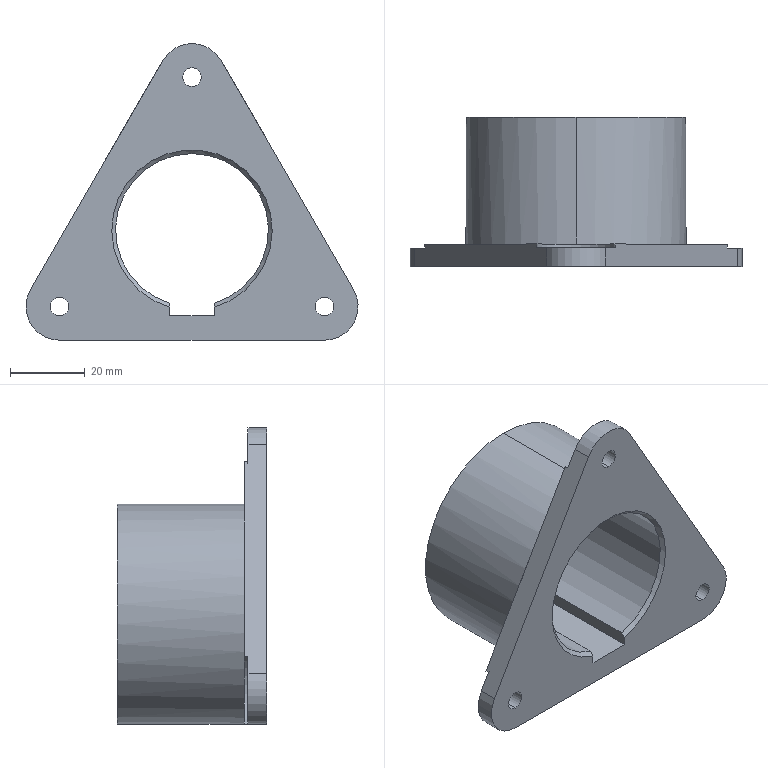Part | SolidWorks | features ICE 2, Chamfer 1, Extrusion 1, HoleWzd 1 | 1 solid | 34 faces | box 89.014 x 40 x 79.5 mm | volume 63655 mm3 | cylinder 17 | plane 14 | cone 3 | commonest cylinder face diameters 5 x6 21 x5 18 x3 59 x2 41 x1
STEP:
#1=CARTESIAN_POINT('',(35.507,5.,-10.));
#2=VERTEX_POINT('',#1);
#3=CARTESIAN_POINT('',(40.597,5.,-11.316));
#4=VERTEX_POINT('',#3);
#5=CARTESIAN_POINT('',(35.507,5.,-20.5));
#6=DIRECTION('',(0.,1.,0.));
#7=DIRECTION('',(0.,0.,1.));
#8=AXIS2_PLACEMENT_3D('',#5,#6,#7);
#9=CIRCLE('',#8,10.5);
#10=EDGE_CURVE('',#2,#4,#9,.T.);
#11=ORIENTED_EDGE('',*,*,#10,.F.);
#12=CARTESIAN_POINT('',(35.507,6.,-10.));
#13=VERTEX_POINT('',#12);
#14=CARTESIAN_POINT('',(35.507,5.,-10.));
#15=DIRECTION('',(0.,1.,0.));
#16=VECTOR('',#15,1000.);
#17=LINE('',#14,#16);
#18=EDGE_CURVE('',#2,#13,#17,.T.);
#19=ORIENTED_EDGE('',*,*,#18,.T.);
#20=CARTESIAN_POINT('',(40.597,6.,-11.316));
#21=VERTEX_POINT('',#20);
#22=CARTESIAN_POINT('',(35.507,6.,-20.5));
#23=DIRECTION('',(0.,1.,0.));
#24=DIRECTION('',(0.,0.,1.));
#25=AXIS2_PLACEMENT_3D('',#22,#23,#24);
#26=CIRCLE('',#25,10.5);
#27=EDGE_CURVE('',#13,#21,#26,.T.);
#28=ORIENTED_EDGE('',*,*,#27,.T.);
#29=CARTESIAN_POINT('',(40.597,5.,-11.316));
#30=DIRECTION('',(0.,-1.,0.));
#31=VECTOR('',#30,1000.);
#32=LINE('',#29,#31);
#33=EDGE_CURVE('',#21,#4,#32,.T.);
#34=ORIENTED_EDGE('',*,*,#33,.T.);
#35=EDGE_LOOP('',(#11,#19,#28,#34));
#36=FACE_OUTER_BOUND('',#35,.T.);
#37=CARTESIAN_POINT('',(35.507,5.,-20.5));
#38=DIRECTION('',(0.,1.,0.));
#39=DIRECTION('',(0.,0.,1.));
#40=AXIS2_PLACEMENT_3D('',#37,#38,#39);
#41=CYLINDRICAL_SURFACE('',#40,10.5);
#42=ADVANCED_FACE('',(#36),#41,.F.);
#43=CARTESIAN_POINT('',(-35.507,5.,-10.));
#44=VERTEX_POINT('',#43);
#45=CARTESIAN_POINT('',(-30.099,5.,-29.5));
#46=VERTEX_POINT('',#45);
#47=CARTESIAN_POINT('',(-35.507,5.,-20.5));
#48=DIRECTION('',(0.,1.,0.));
#49=DIRECTION('',(0.,0.,1.));
#50=AXIS2_PLACEMENT_3D('',#47,#48,#49);
#51=CIRCLE('',#50,10.5);
#52=EDGE_CURVE('',#44,#46,#51,.T.);
#53=ORIENTED_EDGE('',*,*,#52,.F.);
#54=CARTESIAN_POINT('',(-35.507,6.,-10.));
#55=VERTEX_POINT('',#54);
#56=CARTESIAN_POINT('',(-35.507,5.,-10.));
#57=DIRECTION('',(0.,1.,0.));
#58=VECTOR('',#57,1000.);
#59=LINE('',#56,#58);
#60=EDGE_CURVE('',#44,#55,#59,.T.);
#61=ORIENTED_EDGE('',*,*,#60,.T.);
#62=CARTESIAN_POINT('',(-30.099,6.,-29.5));
#63=VERTEX_POINT('',#62);
#64=CARTESIAN_POINT('',(-35.507,6.,-20.5));
#65=DIRECTION('',(0.,1.,0.));
#66=DIRECTION('',(0.,0.,1.));
#67=AXIS2_PLACEMENT_3D('',#64,#65,#66);
#68=CIRCLE('',#67,10.5);
#69=EDGE_CURVE('',#55,#63,#68,.T.);
#70=ORIENTED_EDGE('',*,*,#69,.T.);
#71=CARTESIAN_POINT('',(-30.099,5.,-29.5));
#72=DIRECTION('',(0.,-1.,0.));
#73=VECTOR('',#72,1000.);
#74=LINE('',#71,#73);
#75=EDGE_CURVE('',#63,#46,#74,.T.);
#76=ORIENTED_EDGE('',*,*,#75,.T.);
#77=EDGE_LOOP('',(#53,#61,#70,#76));
#78=FACE_OUTER_BOUND('',#77,.T.);
#79=CARTESIAN_POINT('',(-35.507,5.,-20.5));
#80=DIRECTION('',(0.,1.,0.));
#81=DIRECTION('',(0.,0.,1.));
#82=AXIS2_PLACEMENT_3D('',#79,#80,#81);
#83=CYLINDRICAL_SURFACE('',#82,10.5);
#84=ADVANCED_FACE('',(#78),#83,.F.);
#85=CARTESIAN_POINT('',(0.,39.,20.5));
#86=VERTEX_POINT('',#85);
#87=CARTESIAN_POINT('',(6.,39.,-19.602));
#88=VERTEX_POINT('',#87);
#89=CARTESIAN_POINT('',(0.,39.,0.));
#90=DIRECTION('',(0.,1.,0.));
#91=DIRECTION('',(0.,0.,1.));
#92=AXIS2_PLACEMENT_3D('',#89,#90,#91);
#93=CIRCLE('',#92,20.5);
#94=EDGE_CURVE('',#86,#88,#93,.T.);
#95=ORIENTED_EDGE('',*,*,#94,.F.);
#96=CARTESIAN_POINT('',(0.,40.,21.5));
#97=VERTEX_POINT('',#96);
#98=CARTESIAN_POINT('',(0.,39.,20.5));
#99=DIRECTION('',(0.,0.7071,0.7071));
#100=VECTOR('',#99,1000.);
#101=LINE('',#98,#100);
#102=EDGE_CURVE('',#86,#97,#101,.T.);
#103=ORIENTED_EDGE('',*,*,#102,.T.);
#104=CARTESIAN_POINT('',(6.,40.,-20.646));
#105=VERTEX_POINT('',#104);
#106=CARTESIAN_POINT('',(0.,40.,0.));
#107=DIRECTION('',(0.,-1.,0.));
#108=DIRECTION('',(0.,0.,1.));
#109=AXIS2_PLACEMENT_3D('',#106,#107,#108);
#110=CIRCLE('',#109,21.5);
#111=EDGE_CURVE('',#105,#97,#110,.T.);
#112=ORIENTED_EDGE('',*,*,#111,.F.);
#113=CARTESIAN_POINT('',(6.,39.,-19.602));
#114=CARTESIAN_POINT('',(6.,39.333,-19.95));
#115=CARTESIAN_POINT('',(6.,39.666,-20.298));
#116=CARTESIAN_POINT('',(6.,40.,-20.646));
#117=B_SPLINE_CURVE_WITH_KNOTS('',3,(#113,#114,#115,#116),.UNSPECIFIED.,.F.,.F.,(4,4),(0.,0.001445),.UNSPECIFIED.);
#118=EDGE_CURVE('',#88,#105,#117,.T.);
#119=ORIENTED_EDGE('',*,*,#118,.F.);
#120=EDGE_LOOP('',(#95,#103,#112,#119));
#121=FACE_OUTER_BOUND('',#120,.T.);
#122=CARTESIAN_POINT('',(0.,39.,0.));
#123=DIRECTION('',(0.,1.,0.));
#124=DIRECTION('',(0.,0.,1.));
#125=AXIS2_PLACEMENT_3D('',#122,#123,#124);
#126=CONICAL_SURFACE('',#125,20.5,0.7854);
#127=ADVANCED_FACE('',(#121),#126,.F.);
#128=CARTESIAN_POINT('',(0.,40.,29.5));
#129=VERTEX_POINT('',#128);
#130=CARTESIAN_POINT('',(0.,40.,-29.5));
#131=VERTEX_POINT('',#130);
#132=CARTESIAN_POINT('',(0.,40.,0.));
#133=DIRECTION('',(0.,1.,0.));
#134=DIRECTION('',(0.,0.,1.));
#135=AXIS2_PLACEMENT_3D('',#132,#133,#134);
#136=CIRCLE('',#135,29.5);
#137=EDGE_CURVE('',#129,#131,#136,.T.);
#138=ORIENTED_EDGE('',*,*,#137,.F.);
#139=CARTESIAN_POINT('',(0.,6.,29.5));
#140=VERTEX_POINT('',#139);
#141=CARTESIAN_POINT('',(0.,40.,29.5));
#142=DIRECTION('',(0.,-1.,0.));
#143=VECTOR('',#142,1000.);
#144=LINE('',#141,#143);
#145=EDGE_CURVE('',#129,#140,#144,.T.);
#146=ORIENTED_EDGE('',*,*,#145,.T.);
#147=CARTESIAN_POINT('',(25.548,6.,14.75));
#148=VERTEX_POINT('',#147);
#149=CARTESIAN_POINT('',(0.,6.,0.));
#150=DIRECTION('',(0.,1.,0.));
#151=DIRECTION('',(0.,0.,1.));
#152=AXIS2_PLACEMENT_3D('',#149,#150,#151);
#153=CIRCLE('',#152,29.5);
#154=EDGE_CURVE('',#140,#148,#153,.T.);
#155=ORIENTED_EDGE('',*,*,#154,.T.);
#156=CARTESIAN_POINT('',(0.,6.,-29.5));
#157=VERTEX_POINT('',#156);
#158=CARTESIAN_POINT('',(0.,6.,0.));
#159=DIRECTION('',(0.,1.,0.));
#160=DIRECTION('',(0.,0.,1.));
#161=AXIS2_PLACEMENT_3D('',#158,#159,#160);
#162=CIRCLE('',#161,29.5);
#163=EDGE_CURVE('',#148,#157,#162,.T.);
#164=ORIENTED_EDGE('',*,*,#163,.T.);
#165=CARTESIAN_POINT('',(0.,40.,-29.5));
#166=DIRECTION('',(0.,-1.,0.));
#167=VECTOR('',#166,1000.);
#168=LINE('',#165,#167);
#169=EDGE_CURVE('',#131,#157,#168,.T.);
#170=ORIENTED_EDGE('',*,*,#169,.F.);
#171=EDGE_LOOP('',(#138,#146,#155,#164,#170));
#172=FACE_OUTER_BOUND('',#171,.T.);
#173=CARTESIAN_POINT('',(0.,40.,0.));
#174=DIRECTION('',(0.,-1.,0.));
#175=DIRECTION('',(0.,0.,-1.));
#176=AXIS2_PLACEMENT_3D('',#173,#174,#175);
#177=CYLINDRICAL_SURFACE('',#176,29.5);
#178=ADVANCED_FACE('',(#172),#177,.T.);
#179=CARTESIAN_POINT('',(-35.507,0.,-23.));
#180=VERTEX_POINT('',#179);
#181=CARTESIAN_POINT('',(-35.507,0.,-18.));
#182=VERTEX_POINT('',#181);
#183=CARTESIAN_POINT('',(-35.507,0.,-20.5));
#184=DIRECTION('',(0.,1.,0.));
#185=DIRECTION('',(0.,0.,1.));
#186=AXIS2_PLACEMENT_3D('',#183,#184,#185);
#187=CIRCLE('',#186,2.5);
#188=EDGE_CURVE('',#180,#182,#187,.T.);
#189=ORIENTED_EDGE('',*,*,#188,.F.);
#190=CARTESIAN_POINT('',(-35.507,5.,-23.));
#191=VERTEX_POINT('',#190);
#192=CARTESIAN_POINT('',(-35.507,6.,-23.));
#193=DIRECTION('',(0.,1.,0.));
#194=VECTOR('',#193,1000.);
#195=LINE('',#192,#194);
#196=EDGE_CURVE('',#180,#191,#195,.T.);
#197=ORIENTED_EDGE('',*,*,#196,.T.);
#198=CARTESIAN_POINT('',(-35.507,5.,-18.));
#199=VERTEX_POINT('',#198);
#200=CARTESIAN_POINT('',(-35.507,5.,-20.5));
#201=DIRECTION('',(0.,-1.,0.));
#202=DIRECTION('',(0.,0.,1.));
#203=AXIS2_PLACEMENT_3D('',#200,#201,#202);
#204=CIRCLE('',#203,2.5);
#205=EDGE_CURVE('',#199,#191,#204,.T.);
#206=ORIENTED_EDGE('',*,*,#205,.F.);
#207=CARTESIAN_POINT('',(-35.507,6.,-18.));
#208=DIRECTION('',(0.,1.,0.));
#209=VECTOR('',#208,1000.);
#210=LINE('',#207,#209);
#211=EDGE_CURVE('',#182,#199,#210,.T.);
#212=ORIENTED_EDGE('',*,*,#211,.F.);
#213=EDGE_LOOP('',(#189,#197,#206,#212));
#214=FACE_OUTER_BOUND('',#213,.T.);
#215=CARTESIAN_POINT('',(-35.507,6.,-20.5));
#216=DIRECTION('',(0.,1.,0.));
#217=DIRECTION('',(0.,0.,1.));
#218=AXIS2_PLACEMENT_3D('',#215,#216,#217);
#219=CYLINDRICAL_SURFACE('',#218,2.5);
#220=ADVANCED_FACE('',(#214),#219,.F.);
#221=CARTESIAN_POINT('',(35.507,0.,-23.));
#222=VERTEX_POINT('',#221);
#223=CARTESIAN_POINT('',(35.507,0.,-18.));
#224=VERTEX_POINT('',#223);
#225=CARTESIAN_POINT('',(35.507,0.,-20.5));
#226=DIRECTION('',(0.,1.,0.));
#227=DIRECTION('',(0.,0.,1.));
#228=AXIS2_PLACEMENT_3D('',#225,#226,#227);
#229=CIRCLE('',#228,2.5);
#230=EDGE_CURVE('',#222,#224,#229,.T.);
#231=ORIENTED_EDGE('',*,*,#230,.F.);
#232=CARTESIAN_POINT('',(35.507,5.,-23.));
#233=VERTEX_POINT('',#232);
#234=CARTESIAN_POINT('',(35.507,6.,-23.));
#235=DIRECTION('',(0.,1.,0.));
#236=VECTOR('',#235,1000.);
#237=LINE('',#234,#236);
#238=EDGE_CURVE('',#222,#233,#237,.T.);
#239=ORIENTED_EDGE('',*,*,#238,.T.);
#240=CARTESIAN_POINT('',(35.507,5.,-18.));
#241=VERTEX_POINT('',#240);
#242=CARTESIAN_POINT('',(35.507,5.,-20.5));
#243=DIRECTION('',(0.,-1.,0.));
#244=DIRECTION('',(0.,0.,1.));
#245=AXIS2_PLACEMENT_3D('',#242,#243,#244);
#246=CIRCLE('',#245,2.5);
#247=EDGE_CURVE('',#241,#233,#246,.T.);
#248=ORIENTED_EDGE('',*,*,#247,.F.);
#249=CARTESIAN_POINT('',(35.507,6.,-18.));
#250=DIRECTION('',(0.,1.,0.));
#251=VECTOR('',#250,1000.);
#252=LINE('',#249,#251);
#253=EDGE_CURVE('',#224,#241,#252,.T.);
#254=ORIENTED_EDGE('',*,*,#253,.F.);
#255=EDGE_LOOP('',(#231,#239,#248,#254));
#256=FACE_OUTER_BOUND('',#255,.T.);
#257=CARTESIAN_POINT('',(35.507,6.,-20.5));
#258=DIRECTION('',(0.,1.,0.));
#259=DIRECTION('',(0.,0.,1.));
#260=AXIS2_PLACEMENT_3D('',#257,#258,#259);
#261=CYLINDRICAL_SURFACE('',#260,2.5);
#262=ADVANCED_FACE('',(#256),#261,.F.);
#263=CARTESIAN_POINT('',(0.,0.,38.5));
#264=VERTEX_POINT('',#263);
#265=CARTESIAN_POINT('',(0.,0.,43.5));
#266=VERTEX_POINT('',#265);
#267=CARTESIAN_POINT('',(0.,0.,41.));
#268=DIRECTION('',(0.,1.,0.));
#269=DIRECTION('',(0.,0.,1.));
#270=AXIS2_PLACEMENT_3D('',#267,#268,#269);
#271=CIRCLE('',#270,2.5);
#272=EDGE_CURVE('',#264,#266,#271,.T.);
#273=ORIENTED_EDGE('',*,*,#272,.F.);
#274=CARTESIAN_POINT('',(0.,5.,38.5));
#275=VERTEX_POINT('',#274);
#276=CARTESIAN_POINT('',(0.,6.,38.5));
#277=DIRECTION('',(0.,1.,0.));
#278=VECTOR('',#277,1000.);
#279=LINE('',#276,#278);
#280=EDGE_CURVE('',#264,#275,#279,.T.);
#281=ORIENTED_EDGE('',*,*,#280,.T.);
#282=CARTESIAN_POINT('',(0.,5.,43.5));
#283=VERTEX_POINT('',#282);
#284=CARTESIAN_POINT('',(0.,5.,41.));
#285=DIRECTION('',(0.,-1.,0.));
#286=DIRECTION('',(0.,0.,1.));
#287=AXIS2_PLACEMENT_3D('',#284,#285,#286);
#288=CIRCLE('',#287,2.5);
#289=EDGE_CURVE('',#283,#275,#288,.T.);
#290=ORIENTED_EDGE('',*,*,#289,.F.);
#291=CARTESIAN_POINT('',(0.,6.,43.5));
#292=DIRECTION('',(0.,1.,0.));
#293=VECTOR('',#292,1000.);
#294=LINE('',#291,#293);
#295=EDGE_CURVE('',#266,#283,#294,.T.);
#296=ORIENTED_EDGE('',*,*,#295,.F.);
#297=EDGE_LOOP('',(#273,#281,#290,#296));
#298=FACE_OUTER_BOUND('',#297,.T.);
#299=CARTESIAN_POINT('',(0.,6.,41.));
#300=DIRECTION('',(0.,1.,0.));
#301=DIRECTION('',(0.,0.,1.));
#302=AXIS2_PLACEMENT_3D('',#299,#300,#301);
#303=CYLINDRICAL_SURFACE('',#302,2.5);
#304=ADVANCED_FACE('',(#298),#303,.F.);
#305=CARTESIAN_POINT('',(-7.794,5.,45.5));
#306=VERTEX_POINT('',#305);
#307=CARTESIAN_POINT('',(7.794,5.,45.5));
#308=VERTEX_POINT('',#307);
#309=CARTESIAN_POINT('',(0.,5.,41.));
#310=DIRECTION('',(0.,1.,0.));
#311=DIRECTION('',(0.,0.,1.));
#312=AXIS2_PLACEMENT_3D('',#309,#310,#311);
#313=CIRCLE('',#312,9.);
#314=EDGE_CURVE('',#306,#308,#313,.T.);
#315=ORIENTED_EDGE('',*,*,#314,.F.);
#316=CARTESIAN_POINT('',(-7.794,0.,45.5));
#317=VERTEX_POINT('',#316);
#318=CARTESIAN_POINT('',(-7.794,6.,45.5));
#319=DIRECTION('',(0.,-1.,0.));
#320=VECTOR('',#319,1000.);
#321=LINE('',#318,#320);
#322=EDGE_CURVE('',#306,#317,#321,.T.);
#323=ORIENTED_EDGE('',*,*,#322,.T.);
#324=CARTESIAN_POINT('',(7.794,0.,45.5));
#325=VERTEX_POINT('',#324);
#326=CARTESIAN_POINT('',(0.,0.,41.));
#327=DIRECTION('',(0.,1.,0.));
#328=DIRECTION('',(0.,0.,1.));
#329=AXIS2_PLACEMENT_3D('',#326,#327,#328);
#330=CIRCLE('',#329,9.);
#331=EDGE_CURVE('',#317,#325,#330,.T.);
#332=ORIENTED_EDGE('',*,*,#331,.T.);
#333=CARTESIAN_POINT('',(7.794,6.,45.5));
#334=DIRECTION('',(0.,-1.,0.));
#335=VECTOR('',#334,1000.);
#336=LINE('',#333,#335);
#337=EDGE_CURVE('',#308,#325,#336,.T.);
#338=ORIENTED_EDGE('',*,*,#337,.F.);
#339=EDGE_LOOP('',(#315,#323,#332,#338));
#340=FACE_OUTER_BOUND('',#339,.T.);
#341=CARTESIAN_POINT('',(0.,6.,41.));
#342=DIRECTION('',(0.,-1.,0.));
#343=DIRECTION('',(0.,0.,-1.));
#344=AXIS2_PLACEMENT_3D('',#341,#342,#343);
#345=CYLINDRICAL_SURFACE('',#344,9.);
#346=ADVANCED_FACE('',(#340),#345,.T.);
#347=ORIENTED_EDGE('',*,*,#280,.F.);
#348=CARTESIAN_POINT('',(0.,0.,41.));
#349=DIRECTION('',(0.,1.,0.));
#350=DIRECTION('',(0.,0.,1.));
#351=AXIS2_PLACEMENT_3D('',#348,#349,#350);
#352=CIRCLE('',#351,2.5);
#353=EDGE_CURVE('',#266,#264,#352,.T.);
#354=ORIENTED_EDGE('',*,*,#353,.F.);
#355=ORIENTED_EDGE('',*,*,#295,.T.);
#356=CARTESIAN_POINT('',(0.,5.,41.));
#357=DIRECTION('',(0.,-1.,0.));
#358=DIRECTION('',(0.,0.,1.));
#359=AXIS2_PLACEMENT_3D('',#356,#357,#358);
#360=CIRCLE('',#359,2.5);
#361=EDGE_CURVE('',#275,#283,#360,.T.);
#362=ORIENTED_EDGE('',*,*,#361,.F.);
#363=EDGE_LOOP('',(#347,#354,#355,#362));
#364=FACE_OUTER_BOUND('',#363,.T.);
#365=CARTESIAN_POINT('',(0.,6.,41.));
#366=DIRECTION('',(0.,1.,0.));
#367=DIRECTION('',(0.,0.,1.));
#368=AXIS2_PLACEMENT_3D('',#365,#366,#367);
#369=CYLINDRICAL_SURFACE('',#368,2.5);
#370=ADVANCED_FACE('',(#364),#369,.F.);
#371=CARTESIAN_POINT('',(43.301,5.,-16.));
#372=VERTEX_POINT('',#371);
#373=CARTESIAN_POINT('',(35.507,5.,-29.5));
#374=VERTEX_POINT('',#373);
#375=CARTESIAN_POINT('',(35.507,5.,-20.5));
#376=DIRECTION('',(0.,1.,0.));
#377=DIRECTION('',(0.,0.,1.));
#378=AXIS2_PLACEMENT_3D('',#375,#376,#377);
#379=CIRCLE('',#378,9.);
#380=EDGE_CURVE('',#372,#374,#379,.T.);
#381=ORIENTED_EDGE('',*,*,#380,.F.);
#382=CARTESIAN_POINT('',(43.301,0.,-16.));
#383=VERTEX_POINT('',#382);
#384=CARTESIAN_POINT('',(43.301,6.,-16.));
#385=DIRECTION('',(0.,-1.,0.));
#386=VECTOR('',#385,1000.);
#387=LINE('',#384,#386);
#388=EDGE_CURVE('',#372,#383,#387,.T.);
#389=ORIENTED_EDGE('',*,*,#388,.T.);
#390=CARTESIAN_POINT('',(35.507,0.,-29.5));
#391=VERTEX_POINT('',#390);
#392=CARTESIAN_POINT('',(35.507,0.,-20.5));
#393=DIRECTION('',(0.,1.,0.));
#394=DIRECTION('',(0.,0.,1.));
#395=AXIS2_PLACEMENT_3D('',#392,#393,#394);
#396=CIRCLE('',#395,9.);
#397=EDGE_CURVE('',#383,#391,#396,.T.);
#398=ORIENTED_EDGE('',*,*,#397,.T.);
#399=CARTESIAN_POINT('',(35.507,6.,-29.5));
#400=DIRECTION('',(0.,-1.,0.));
#401=VECTOR('',#400,1000.);
#402=LINE('',#399,#401);
#403=EDGE_CURVE('',#374,#391,#402,.T.);
#404=ORIENTED_EDGE('',*,*,#403,.F.);
#405=EDGE_LOOP('',(#381,#389,#398,#404));
#406=FACE_OUTER_BOUND('',#405,.T.);
#407=CARTESIAN_POINT('',(35.507,6.,-20.5));
#408=DIRECTION('',(0.,-1.,0.));
#409=DIRECTION('',(0.,0.,-1.));
#410=AXIS2_PLACEMENT_3D('',#407,#408,#409);
#411=CYLINDRICAL_SURFACE('',#410,9.);
#412=ADVANCED_FACE('',(#406),#411,.T.);
#413=ORIENTED_EDGE('',*,*,#238,.F.);
#414=CARTESIAN_POINT('',(35.507,0.,-20.5));
#415=DIRECTION('',(0.,1.,0.));
#416=DIRECTION('',(0.,0.,1.));
#417=AXIS2_PLACEMENT_3D('',#414,#415,#416);
#418=CIRCLE('',#417,2.5);
#419=EDGE_CURVE('',#224,#222,#418,.T.);
#420=ORIENTED_EDGE('',*,*,#419,.F.);
#421=ORIENTED_EDGE('',*,*,#253,.T.);
#422=CARTESIAN_POINT('',(35.507,5.,-20.5));
#423=DIRECTION('',(0.,-1.,0.));
#424=DIRECTION('',(0.,0.,1.));
#425=AXIS2_PLACEMENT_3D('',#422,#423,#424);
#426=CIRCLE('',#425,2.5);
#427=EDGE_CURVE('',#233,#241,#426,.T.);
#428=ORIENTED_EDGE('',*,*,#427,.F.);
#429=EDGE_LOOP('',(#413,#420,#421,#428));
#430=FACE_OUTER_BOUND('',#429,.T.);
#431=CARTESIAN_POINT('',(35.507,6.,-20.5));
#432=DIRECTION('',(0.,1.,0.));
#433=DIRECTION('',(0.,0.,1.));
#434=AXIS2_PLACEMENT_3D('',#431,#432,#433);
#435=CYLINDRICAL_SURFACE('',#434,2.5);
#436=ADVANCED_FACE('',(#430),#435,.F.);
#437=CARTESIAN_POINT('',(-35.507,5.,-29.5));
#438=VERTEX_POINT('',#437);
#439=CARTESIAN_POINT('',(-43.301,5.,-16.));
#440=VERTEX_POINT('',#439);
#441=CARTESIAN_POINT('',(-35.507,5.,-20.5));
#442=DIRECTION('',(0.,1.,0.));
#443=DIRECTION('',(0.,0.,1.));
#444=AXIS2_PLACEMENT_3D('',#441,#442,#443);
#445=CIRCLE('',#444,9.);
#446=EDGE_CURVE('',#438,#440,#445,.T.);
#447=ORIENTED_EDGE('',*,*,#446,.F.);
#448=CARTESIAN_POINT('',(-35.507,0.,-29.5));
#449=VERTEX_POINT('',#448);
#450=CARTESIAN_POINT('',(-35.507,6.,-29.5));
#451=DIRECTION('',(0.,-1.,0.));
#452=VECTOR('',#451,1000.);
#453=LINE('',#450,#452);
#454=EDGE_CURVE('',#438,#449,#453,.T.);
#455=ORIENTED_EDGE('',*,*,#454,.T.);
#456=CARTESIAN_POINT('',(-43.301,0.,-16.));
#457=VERTEX_POINT('',#456);
#458=CARTESIAN_POINT('',(-35.507,0.,-20.5));
#459=DIRECTION('',(0.,1.,0.));
#460=DIRECTION('',(0.,0.,1.));
#461=AXIS2_PLACEMENT_3D('',#458,#459,#460);
#462=CIRCLE('',#461,9.);
#463=EDGE_CURVE('',#449,#457,#462,.T.);
#464=ORIENTED_EDGE('',*,*,#463,.T.);
#465=CARTESIAN_POINT('',(-43.301,6.,-16.));
#466=DIRECTION('',(0.,-1.,0.));
#467=VECTOR('',#466,1000.);
#468=LINE('',#465,#467);
#469=EDGE_CURVE('',#440,#457,#468,.T.);
#470=ORIENTED_EDGE('',*,*,#469,.F.);
#471=EDGE_LOOP('',(#447,#455,#464,#470));
#472=FACE_OUTER_BOUND('',#471,.T.);
#473=CARTESIAN_POINT('',(-35.507,6.,-20.5));
#474=DIRECTION('',(0.,-1.,0.));
#475=DIRECTION('',(0.,0.,-1.));
#476=AXIS2_PLACEMENT_3D('',#473,#474,#475);
#477=CYLINDRICAL_SURFACE('',#476,9.);
#478=ADVANCED_FACE('',(#472),#477,.T.);
#479=ORIENTED_EDGE('',*,*,#196,.F.);
#480=CARTESIAN_POINT('',(-35.507,0.,-20.5));
#481=DIRECTION('',(0.,1.,0.));
#482=DIRECTION('',(0.,0.,1.));
#483=AXIS2_PLACEMENT_3D('',#480,#481,#482);
#484=CIRCLE('',#483,2.5);
#485=EDGE_CURVE('',#182,#180,#484,.T.);
#486=ORIENTED_EDGE('',*,*,#485,.F.);
#487=ORIENTED_EDGE('',*,*,#211,.T.);
#488=CARTESIAN_POINT('',(-35.507,5.,-20.5));
#489=DIRECTION('',(0.,-1.,0.));
#490=DIRECTION('',(0.,0.,1.));
#491=AXIS2_PLACEMENT_3D('',#488,#489,#490);
#492=CIRCLE('',#491,2.5);
#493=EDGE_CURVE('',#191,#199,#492,.T.);
#494=ORIENTED_EDGE('',*,*,#493,.F.);
#495=EDGE_LOOP('',(#479,#486,#487,#494));
#496=FACE_OUTER_BOUND('',#495,.T.);
#497=CARTESIAN_POINT('',(-35.507,6.,-20.5));
#498=DIRECTION('',(0.,1.,0.));
#499=DIRECTION('',(0.,0.,1.));
#500=AXIS2_PLACEMENT_3D('',#497,#498,#499);
#501=CYLINDRICAL_SURFACE('',#500,2.5);
#502=ADVANCED_FACE('',(#496),#501,.F.);
#503=CARTESIAN_POINT('',(30.099,5.,-29.5));
#504=VERTEX_POINT('',#503);
#505=CARTESIAN_POINT('',(30.099,6.,-29.5));
#506=VERTEX_POINT('',#505);
#507=CARTESIAN_POINT('',(30.099,5.,-29.5));
#508=DIRECTION('',(0.,1.,0.));
#509=VECTOR('',#508,1000.);
#510=LINE('',#507,#509);
#511=EDGE_CURVE('',#504,#506,#510,.T.);
#512=ORIENTED_EDGE('',*,*,#511,.F.);
#513=CARTESIAN_POINT('',(0.,5.,-29.5));
#514=DIRECTION('',(1.,0.,0.));
#515=VECTOR('',#514,1000.);
#516=LINE('',#513,#515);
#517=EDGE_CURVE('',#504,#374,#516,.T.);
#518=ORIENTED_EDGE('',*,*,#517,.T.);
#519=ORIENTED_EDGE('',*,*,#403,.T.);
#520=CARTESIAN_POINT('',(0.,0.,-29.5));
#521=DIRECTION('',(1.,0.,0.));
#522=VECTOR('',#521,1000.);
#523=LINE('',#520,#522);
#524=EDGE_CURVE('',#449,#391,#523,.T.);
#525=ORIENTED_EDGE('',*,*,#524,.F.);
#526=ORIENTED_EDGE('',*,*,#454,.F.);
#527=CARTESIAN_POINT('',(0.,5.,-29.5));
#528=DIRECTION('',(1.,0.,0.));
#529=VECTOR('',#528,1000.);
#530=LINE('',#527,#529);
#531=EDGE_CURVE('',#438,#46,#530,.T.);
#532=ORIENTED_EDGE('',*,*,#531,.T.);
#533=ORIENTED_EDGE('',*,*,#75,.F.);
#534=CARTESIAN_POINT('',(0.,6.,-29.5));
#535=DIRECTION('',(1.,0.,0.));
#536=VECTOR('',#535,1000.);
#537=LINE('',#534,#536);
#538=EDGE_CURVE('',#63,#157,#537,.T.);
#539=ORIENTED_EDGE('',*,*,#538,.T.);
#540=CARTESIAN_POINT('',(0.,6.,-29.5));
#541=DIRECTION('',(1.,0.,0.));
#542=VECTOR('',#541,1000.);
#543=LINE('',#540,#542);
#544=EDGE_CURVE('',#157,#506,#543,.T.);
#545=ORIENTED_EDGE('',*,*,#544,.T.);
#546=EDGE_LOOP('',(#512,#518,#519,#525,#526,#532,#533,#539,#545));
#547=FACE_OUTER_BOUND('',#546,.T.);
#548=CARTESIAN_POINT('',(0.,6.,-29.5));
#549=DIRECTION('',(0.,0.,-1.));
#550=DIRECTION('',(-1.,0.,0.));
#551=AXIS2_PLACEMENT_3D('',#548,#549,#550);
#552=PLANE('',#551);
#553=ADVANCED_FACE('',(#547),#552,.T.);
#554=CARTESIAN_POINT('',(-10.498,6.,40.816));
#555=VERTEX_POINT('',#554);
#556=CARTESIAN_POINT('',(-10.498,5.,40.816));
#557=VERTEX_POINT('',#556);
#558=CARTESIAN_POINT('',(-10.498,5.,40.816));
#559=DIRECTION('',(0.,-1.,0.));
#560=VECTOR('',#559,1000.);
#561=LINE('',#558,#560);
#562=EDGE_CURVE('',#555,#557,#561,.T.);
#563=ORIENTED_EDGE('',*,*,#562,.F.);
#564=CARTESIAN_POINT('',(-25.548,6.,14.75));
#565=VERTEX_POINT('',#564);
#566=CARTESIAN_POINT('',(-25.548,6.,14.75));
#567=DIRECTION('',(-0.5,0.,-0.866));
#568=VECTOR('',#567,1000.);
#569=LINE('',#566,#568);
#570=EDGE_CURVE('',#555,#565,#569,.T.);
#571=ORIENTED_EDGE('',*,*,#570,.T.);
#572=CARTESIAN_POINT('',(-40.597,6.,-11.316));
#573=VERTEX_POINT('',#572);
#574=CARTESIAN_POINT('',(-25.548,6.,14.75));
#575=DIRECTION('',(-0.5,0.,-0.866));
#576=VECTOR('',#575,1000.);
#577=LINE('',#574,#576);
#578=EDGE_CURVE('',#565,#573,#577,.T.);
#579=ORIENTED_EDGE('',*,*,#578,.T.);
#580=CARTESIAN_POINT('',(-40.597,5.,-11.316));
#581=VERTEX_POINT('',#580);
#582=CARTESIAN_POINT('',(-40.597,5.,-11.316));
#583=DIRECTION('',(0.,1.,0.));
#584=VECTOR('',#583,1000.);
#585=LINE('',#582,#584);
#586=EDGE_CURVE('',#581,#573,#585,.T.);
#587=ORIENTED_EDGE('',*,*,#586,.F.);
#588=CARTESIAN_POINT('',(-25.548,5.,14.75));
#589=DIRECTION('',(-0.5,0.,-0.866));
#590=VECTOR('',#589,1000.);
#591=LINE('',#588,#590);
#592=EDGE_CURVE('',#581,#440,#591,.T.);
#593=ORIENTED_EDGE('',*,*,#592,.T.);
#594=ORIENTED_EDGE('',*,*,#469,.T.);
#595=CARTESIAN_POINT('',(-25.548,0.,14.75));
#596=DIRECTION('',(-0.5,0.,-0.866));
#597=VECTOR('',#596,1000.);
#598=LINE('',#595,#597);
#599=EDGE_CURVE('',#317,#457,#598,.T.);
#600=ORIENTED_EDGE('',*,*,#599,.F.);
#601=ORIENTED_EDGE('',*,*,#322,.F.);
#602=CARTESIAN_POINT('',(-25.548,5.,14.75));
#603=DIRECTION('',(-0.5,0.,-0.866));
#604=VECTOR('',#603,1000.);
#605=LINE('',#602,#604);
#606=EDGE_CURVE('',#306,#557,#605,.T.);
#607=ORIENTED_EDGE('',*,*,#606,.T.);
#608=EDGE_LOOP('',(#563,#571,#579,#587,#593,#594,#600,#601,#607));
#609=FACE_OUTER_BOUND('',#608,.T.);
#610=CARTESIAN_POINT('',(-25.548,6.,14.75));
#611=DIRECTION('',(-0.866,0.,0.5));
#612=DIRECTION('',(0.5,0.,0.866));
#613=AXIS2_PLACEMENT_3D('',#610,#611,#612);
#614=PLANE('',#613);
#615=ADVANCED_FACE('',(#609),#614,.T.);
#616=CARTESIAN_POINT('',(-35.507,6.,-20.5));
#617=DIRECTION('',(0.,1.,0.));
#618=DIRECTION('',(0.,0.,1.));
#619=AXIS2_PLACEMENT_3D('',#616,#617,#618);
#620=CIRCLE('',#619,10.5);
#621=EDGE_CURVE('',#573,#55,#620,.T.);
#622=ORIENTED_EDGE('',*,*,#621,.F.);
#623=ORIENTED_EDGE('',*,*,#578,.F.);
#624=CARTESIAN_POINT('',(0.,6.,0.));
#625=DIRECTION('',(0.,1.,0.));
#626=DIRECTION('',(0.,0.,1.));
#627=AXIS2_PLACEMENT_3D('',#624,#625,#626);
#628=CIRCLE('',#627,29.5);
#629=EDGE_CURVE('',#157,#565,#628,.T.);
#630=ORIENTED_EDGE('',*,*,#629,.F.);
#631=ORIENTED_EDGE('',*,*,#538,.F.);
#632=ORIENTED_EDGE('',*,*,#69,.F.);
#633=EDGE_LOOP('',(#622,#623,#630,#631,#632));
#634=FACE_OUTER_BOUND('',#633,.T.);
#635=CARTESIAN_POINT('',(0.,6.,0.));
#636=DIRECTION('',(0.,1.,0.));
#637=DIRECTION('',(0.,0.,1.));
#638=AXIS2_PLACEMENT_3D('',#635,#636,#637);
#639=PLANE('',#638);
#640=ADVANCED_FACE('',(#634),#639,.T.);
#641=ORIENTED_EDGE('',*,*,#485,.T.);
#642=ORIENTED_EDGE('',*,*,#188,.T.);
#643=EDGE_LOOP('',(#641,#642));
#644=FACE_BOUND('',#643,.T.);
#645=ORIENTED_EDGE('',*,*,#419,.T.);
#646=ORIENTED_EDGE('',*,*,#230,.T.);
#647=EDGE_LOOP('',(#645,#646));
#648=FACE_BOUND('',#647,.T.);
#649=ORIENTED_EDGE('',*,*,#353,.T.);
#650=ORIENTED_EDGE('',*,*,#272,.T.);
#651=EDGE_LOOP('',(#649,#650));
#652=FACE_BOUND('',#651,.T.);
#653=ORIENTED_EDGE('',*,*,#524,.T.);
#654=ORIENTED_EDGE('',*,*,#397,.F.);
#655=CARTESIAN_POINT('',(25.548,0.,14.75));
#656=DIRECTION('',(-0.5,0.,0.866));
#657=VECTOR('',#656,1000.);
#658=LINE('',#655,#657);
#659=EDGE_CURVE('',#383,#325,#658,.T.);
#660=ORIENTED_EDGE('',*,*,#659,.T.);
#661=ORIENTED_EDGE('',*,*,#331,.F.);
#662=ORIENTED_EDGE('',*,*,#599,.T.);
#663=ORIENTED_EDGE('',*,*,#463,.F.);
#664=EDGE_LOOP('',(#653,#654,#660,#661,#662,#663));
#665=FACE_OUTER_BOUND('',#664,.T.);
#666=CARTESIAN_POINT('',(-6.,0.,-22.902));
#667=VERTEX_POINT('',#666);
#668=CARTESIAN_POINT('',(-6.,0.,-20.646));
#669=VERTEX_POINT('',#668);
#670=CARTESIAN_POINT('',(-6.,0.,-22.902));
#671=DIRECTION('',(0.,0.,1.));
#672=VECTOR('',#671,1000.);
#673=LINE('',#670,#672);
#674=EDGE_CURVE('',#667,#669,#673,.T.);
#675=ORIENTED_EDGE('',*,*,#674,.T.);
#676=CARTESIAN_POINT('',(6.,0.,-20.646));
#677=VERTEX_POINT('',#676);
#678=CARTESIAN_POINT('',(0.,0.,0.));
#679=DIRECTION('',(0.,1.,0.));
#680=DIRECTION('',(0.,0.,1.));
#681=AXIS2_PLACEMENT_3D('',#678,#679,#680);
#682=CIRCLE('',#681,21.5);
#683=EDGE_CURVE('',#669,#677,#682,.T.);
#684=ORIENTED_EDGE('',*,*,#683,.T.);
#685=CARTESIAN_POINT('',(6.,0.,-22.902));
#686=VERTEX_POINT('',#685);
#687=CARTESIAN_POINT('',(6.,0.,-19.602));
#688=DIRECTION('',(0.,0.,-1.));
#689=VECTOR('',#688,1000.);
#690=LINE('',#687,#689);
#691=EDGE_CURVE('',#677,#686,#690,.T.);
#692=ORIENTED_EDGE('',*,*,#691,.T.);
#693=CARTESIAN_POINT('',(6.,0.,-22.902));
#694=DIRECTION('',(-1.,0.,0.));
#695=VECTOR('',#694,1000.);
#696=LINE('',#693,#695);
#697=EDGE_CURVE('',#686,#667,#696,.T.);
#698=ORIENTED_EDGE('',*,*,#697,.T.);
#699=EDGE_LOOP('',(#675,#684,#692,#698));
#700=FACE_BOUND('',#699,.T.);
#701=CARTESIAN_POINT('',(0.,0.,0.));
#702=DIRECTION('',(0.,1.,0.));
#703=DIRECTION('',(0.,0.,1.));
#704=AXIS2_PLACEMENT_3D('',#701,#702,#703);
#705=PLANE('',#704);
#706=ADVANCED_FACE('',(#644,#648,#652,#665,#700),#705,.F.);
#707=ORIENTED_EDGE('',*,*,#145,.F.);
#708=CARTESIAN_POINT('',(0.,40.,0.));
#709=DIRECTION('',(0.,1.,0.));
#710=DIRECTION('',(0.,0.,1.));
#711=AXIS2_PLACEMENT_3D('',#708,#709,#710);
#712=CIRCLE('',#711,29.5);
#713=EDGE_CURVE('',#131,#129,#712,.T.);
#714=ORIENTED_EDGE('',*,*,#713,.F.);
#715=ORIENTED_EDGE('',*,*,#169,.T.);
#716=ORIENTED_EDGE('',*,*,#629,.T.);
#717=CARTESIAN_POINT('',(0.,6.,0.));
#718=DIRECTION('',(0.,1.,0.));
#719=DIRECTION('',(0.,0.,1.));
#720=AXIS2_PLACEMENT_3D('',#717,#718,#719);
#721=CIRCLE('',#720,29.5);
#722=EDGE_CURVE('',#565,#140,#721,.T.);
#723=ORIENTED_EDGE('',*,*,#722,.T.);
#724=EDGE_LOOP('',(#707,#714,#715,#716,#723));
#725=FACE_OUTER_BOUND('',#724,.T.);
#726=CARTESIAN_POINT('',(0.,40.,0.));
#727=DIRECTION('',(0.,-1.,0.));
#728=DIRECTION('',(0.,0.,-1.));
#729=AXIS2_PLACEMENT_3D('',#726,#727,#728);
#730=CYLINDRICAL_SURFACE('',#729,29.5);
#731=ADVANCED_FACE('',(#725),#730,.T.);
#732=ORIENTED_EDGE('',*,*,#713,.T.);
#733=ORIENTED_EDGE('',*,*,#137,.T.);
#734=EDGE_LOOP('',(#732,#733));
#735=FACE_OUTER_BOUND('',#734,.T.);
#736=CARTESIAN_POINT('',(6.,40.,-22.902));
#737=VERTEX_POINT('',#736);
#738=CARTESIAN_POINT('',(6.,40.,-19.602));
#739=DIRECTION('',(0.,0.,-1.));
#740=VECTOR('',#739,1000.);
#741=LINE('',#738,#740);
#742=EDGE_CURVE('',#105,#737,#741,.T.);
#743=ORIENTED_EDGE('',*,*,#742,.F.);
#744=ORIENTED_EDGE('',*,*,#111,.T.);
#745=CARTESIAN_POINT('',(-6.,40.,-20.646));
#746=VERTEX_POINT('',#745);
#747=CARTESIAN_POINT('',(0.,40.,0.));
#748=DIRECTION('',(0.,-1.,0.));
#749=DIRECTION('',(0.,0.,1.));
#750=AXIS2_PLACEMENT_3D('',#747,#748,#749);
#751=CIRCLE('',#750,21.5);
#752=EDGE_CURVE('',#97,#746,#751,.T.);
#753=ORIENTED_EDGE('',*,*,#752,.T.);
#754=CARTESIAN_POINT('',(-6.,40.,-22.902));
#755=VERTEX_POINT('',#754);
#756=CARTESIAN_POINT('',(-6.,40.,-22.902));
#757=DIRECTION('',(0.,0.,1.));
#758=VECTOR('',#757,1000.);
#759=LINE('',#756,#758);
#760=EDGE_CURVE('',#755,#746,#759,.T.);
#761=ORIENTED_EDGE('',*,*,#760,.F.);
#762=CARTESIAN_POINT('',(6.,40.,-22.902));
#763=DIRECTION('',(-1.,0.,0.));
#764=VECTOR('',#763,1000.);
#765=LINE('',#762,#764);
#766=EDGE_CURVE('',#737,#755,#765,.T.);
#767=ORIENTED_EDGE('',*,*,#766,.F.);
#768=EDGE_LOOP('',(#743,#744,#753,#761,#767));
#769=FACE_BOUND('',#768,.T.);
#770=CARTESIAN_POINT('',(0.,40.,0.));
#771=DIRECTION('',(0.,1.,0.));
#772=DIRECTION('',(0.,0.,1.));
#773=AXIS2_PLACEMENT_3D('',#770,#771,#772);
#774=PLANE('',#773);
#775=ADVANCED_FACE('',(#735,#769),#774,.T.);
#776=ORIENTED_EDGE('',*,*,#697,.F.);
#777=CARTESIAN_POINT('',(6.,40.,-22.902));
#778=DIRECTION('',(0.,-1.,0.));
#779=VECTOR('',#778,1000.);
#780=LINE('',#777,#779);
#781=EDGE_CURVE('',#737,#686,#780,.T.);
#782=ORIENTED_EDGE('',*,*,#781,.F.);
#783=ORIENTED_EDGE('',*,*,#766,.T.);
#784=CARTESIAN_POINT('',(-6.,40.,-22.902));
#785=DIRECTION('',(0.,-1.,0.));
#786=VECTOR('',#785,1000.);
#787=LINE('',#784,#786);
#788=EDGE_CURVE('',#755,#667,#787,.T.);
#789=ORIENTED_EDGE('',*,*,#788,.T.);
#790=EDGE_LOOP('',(#776,#782,#783,#789));
#791=FACE_OUTER_BOUND('',#790,.T.);
#792=CARTESIAN_POINT('',(6.,40.,-22.902));
#793=DIRECTION('',(0.,0.,1.));
#794=DIRECTION('',(1.,0.,0.));
#795=AXIS2_PLACEMENT_3D('',#792,#793,#794);
#796=PLANE('',#795);
#797=ADVANCED_FACE('',(#791),#796,.T.);
#798=CARTESIAN_POINT('',(-6.,39.,-19.602));
#799=VERTEX_POINT('',#798);
#800=CARTESIAN_POINT('',(-6.,1.,-19.602));
#801=VERTEX_POINT('',#800);
#802=CARTESIAN_POINT('',(-6.,40.,-19.602));
#803=DIRECTION('',(0.,-1.,0.));
#804=VECTOR('',#803,1000.);
#805=LINE('',#802,#804);
#806=EDGE_CURVE('',#799,#801,#805,.T.);
#807=ORIENTED_EDGE('',*,*,#806,.T.);
#808=CARTESIAN_POINT('',(-6.,1.,-19.602));
#809=CARTESIAN_POINT('',(-6.,0.667,-19.95));
#810=CARTESIAN_POINT('',(-6.,0.3337,-20.298));
#811=CARTESIAN_POINT('',(-6.,0.,-20.646));
#812=B_SPLINE_CURVE_WITH_KNOTS('',3,(#808,#809,#810,#811),.UNSPECIFIED.,.F.,.F.,(4,4),(0.,0.001445),.UNSPECIFIED.);
#813=EDGE_CURVE('',#801,#669,#812,.T.);
#814=ORIENTED_EDGE('',*,*,#813,.T.);
#815=ORIENTED_EDGE('',*,*,#674,.F.);
#816=ORIENTED_EDGE('',*,*,#788,.F.);
#817=ORIENTED_EDGE('',*,*,#760,.T.);
#818=CARTESIAN_POINT('',(-6.,40.,-20.646));
#819=CARTESIAN_POINT('',(-6.,39.666,-20.298));
#820=CARTESIAN_POINT('',(-6.,39.333,-19.95));
#821=CARTESIAN_POINT('',(-6.,39.,-19.602));
#822=B_SPLINE_CURVE_WITH_KNOTS('',3,(#818,#819,#820,#821),.UNSPECIFIED.,.F.,.F.,(4,4),(0.,0.001445),.UNSPECIFIED.);
#823=EDGE_CURVE('',#746,#799,#822,.T.);
#824=ORIENTED_EDGE('',*,*,#823,.T.);
#825=EDGE_LOOP('',(#807,#814,#815,#816,#817,#824));
#826=FACE_OUTER_BOUND('',#825,.T.);
#827=CARTESIAN_POINT('',(-6.,40.,-22.902));
#828=DIRECTION('',(1.,0.,0.));
#829=DIRECTION('',(0.,0.,-1.));
#830=AXIS2_PLACEMENT_3D('',#827,#828,#829);
#831=PLANE('',#830);
#832=ADVANCED_FACE('',(#826),#831,.T.);
#833=CARTESIAN_POINT('',(6.,1.,-19.602));
#834=VERTEX_POINT('',#833);
#835=CARTESIAN_POINT('',(6.,40.,-19.602));
#836=DIRECTION('',(0.,-1.,0.));
#837=VECTOR('',#836,1000.);
#838=LINE('',#835,#837);
#839=EDGE_CURVE('',#88,#834,#838,.T.);
#840=ORIENTED_EDGE('',*,*,#839,.T.);
#841=CARTESIAN_POINT('',(0.,1.,0.));
#842=DIRECTION('',(0.,-1.,0.));
#843=DIRECTION('',(0.,0.,1.));
#844=AXIS2_PLACEMENT_3D('',#841,#842,#843);
#845=CIRCLE('',#844,20.5);
#846=EDGE_CURVE('',#834,#801,#845,.T.);
#847=ORIENTED_EDGE('',*,*,#846,.T.);
#848=ORIENTED_EDGE('',*,*,#806,.F.);
#849=CARTESIAN_POINT('',(0.,39.,0.));
#850=DIRECTION('',(0.,1.,0.));
#851=DIRECTION('',(0.,0.,1.));
#852=AXIS2_PLACEMENT_3D('',#849,#850,#851);
#853=CIRCLE('',#852,20.5);
#854=EDGE_CURVE('',#799,#86,#853,.T.);
#855=ORIENTED_EDGE('',*,*,#854,.T.);
#856=ORIENTED_EDGE('',*,*,#94,.T.);
#857=EDGE_LOOP('',(#840,#847,#848,#855,#856));
#858=FACE_OUTER_BOUND('',#857,.T.);
#859=CARTESIAN_POINT('',(0.,40.,0.));
#860=DIRECTION('',(0.,-1.,0.));
#861=DIRECTION('',(0.,0.,-1.));
#862=AXIS2_PLACEMENT_3D('',#859,#860,#861);
#863=CYLINDRICAL_SURFACE('',#862,20.5);
#864=ADVANCED_FACE('',(#858),#863,.F.);
#865=ORIENTED_EDGE('',*,*,#691,.F.);
#866=CARTESIAN_POINT('',(6.,0.,-20.646));
#867=CARTESIAN_POINT('',(6.,0.3337,-20.298));
#868=CARTESIAN_POINT('',(6.,0.667,-19.95));
#869=CARTESIAN_POINT('',(6.,1.,-19.602));
#870=B_SPLINE_CURVE_WITH_KNOTS('',3,(#866,#867,#868,#869),.UNSPECIFIED.,.F.,.F.,(4,4),(0.,0.001445),.UNSPECIFIED.);
#871=EDGE_CURVE('',#677,#834,#870,.T.);
#872=ORIENTED_EDGE('',*,*,#871,.T.);
#873=ORIENTED_EDGE('',*,*,#839,.F.);
#874=ORIENTED_EDGE('',*,*,#118,.T.);
#875=ORIENTED_EDGE('',*,*,#742,.T.);
#876=ORIENTED_EDGE('',*,*,#781,.T.);
#877=EDGE_LOOP('',(#865,#872,#873,#874,#875,#876));
#878=FACE_OUTER_BOUND('',#877,.T.);
#879=CARTESIAN_POINT('',(6.,40.,-19.602));
#880=DIRECTION('',(-1.,0.,0.));
#881=DIRECTION('',(0.,0.,1.));
#882=AXIS2_PLACEMENT_3D('',#879,#880,#881);
#883=PLANE('',#882);
#884=ADVANCED_FACE('',(#878),#883,.T.);
#885=CARTESIAN_POINT('',(10.498,5.,40.816));
#886=VERTEX_POINT('',#885);
#887=CARTESIAN_POINT('',(10.498,6.,40.816));
#888=VERTEX_POINT('',#887);
#889=CARTESIAN_POINT('',(10.498,5.,40.816));
#890=DIRECTION('',(0.,1.,0.));
#891=VECTOR('',#890,1000.);
#892=LINE('',#889,#891);
#893=EDGE_CURVE('',#886,#888,#892,.T.);
#894=ORIENTED_EDGE('',*,*,#893,.F.);
#895=CARTESIAN_POINT('',(25.548,5.,14.75));
#896=DIRECTION('',(-0.5,0.,0.866));
#897=VECTOR('',#896,1000.);
#898=LINE('',#895,#897);
#899=EDGE_CURVE('',#886,#308,#898,.T.);
#900=ORIENTED_EDGE('',*,*,#899,.T.);
#901=ORIENTED_EDGE('',*,*,#337,.T.);
#902=ORIENTED_EDGE('',*,*,#659,.F.);
#903=ORIENTED_EDGE('',*,*,#388,.F.);
#904=CARTESIAN_POINT('',(25.548,5.,14.75));
#905=DIRECTION('',(-0.5,0.,0.866));
#906=VECTOR('',#905,1000.);
#907=LINE('',#904,#906);
#908=EDGE_CURVE('',#372,#4,#907,.T.);
#909=ORIENTED_EDGE('',*,*,#908,.T.);
#910=ORIENTED_EDGE('',*,*,#33,.F.);
#911=CARTESIAN_POINT('',(25.548,6.,14.75));
#912=DIRECTION('',(-0.5,0.,0.866));
#913=VECTOR('',#912,1000.);
#914=LINE('',#911,#913);
#915=EDGE_CURVE('',#21,#148,#914,.T.);
#916=ORIENTED_EDGE('',*,*,#915,.T.);
#917=CARTESIAN_POINT('',(25.548,6.,14.75));
#918=DIRECTION('',(-0.5,0.,0.866));
#919=VECTOR('',#918,1000.);
#920=LINE('',#917,#919);
#921=EDGE_CURVE('',#148,#888,#920,.T.);
#922=ORIENTED_EDGE('',*,*,#921,.T.);
#923=EDGE_LOOP('',(#894,#900,#901,#902,#903,#909,#910,#916,#922));
#924=FACE_OUTER_BOUND('',#923,.T.);
#925=CARTESIAN_POINT('',(25.548,6.,14.75));
#926=DIRECTION('',(0.866,0.,0.5));
#927=DIRECTION('',(0.5,0.,-0.866));
#928=AXIS2_PLACEMENT_3D('',#925,#926,#927);
#929=PLANE('',#928);
#930=ADVANCED_FACE('',(#924),#929,.T.);
#931=CARTESIAN_POINT('',(0.,6.,41.));
#932=DIRECTION('',(0.,1.,0.));
#933=DIRECTION('',(0.,0.,1.));
#934=AXIS2_PLACEMENT_3D('',#931,#932,#933);
#935=CIRCLE('',#934,10.5);
#936=EDGE_CURVE('',#888,#555,#935,.T.);
#937=ORIENTED_EDGE('',*,*,#936,.F.);
#938=ORIENTED_EDGE('',*,*,#921,.F.);
#939=ORIENTED_EDGE('',*,*,#154,.F.);
#940=ORIENTED_EDGE('',*,*,#722,.F.);
#941=ORIENTED_EDGE('',*,*,#570,.F.);
#942=EDGE_LOOP('',(#937,#938,#939,#940,#941));
#943=FACE_OUTER_BOUND('',#942,.T.);
#944=CARTESIAN_POINT('',(0.,6.,0.));
#945=DIRECTION('',(0.,1.,0.));
#946=DIRECTION('',(0.,0.,1.));
#947=AXIS2_PLACEMENT_3D('',#944,#945,#946);
#948=PLANE('',#947);
#949=ADVANCED_FACE('',(#943),#948,.T.);
#950=CARTESIAN_POINT('',(35.507,6.,-20.5));
#951=DIRECTION('',(0.,1.,0.));
#952=DIRECTION('',(0.,0.,1.));
#953=AXIS2_PLACEMENT_3D('',#950,#951,#952);
#954=CIRCLE('',#953,10.5);
#955=EDGE_CURVE('',#506,#13,#954,.T.);
#956=ORIENTED_EDGE('',*,*,#955,.F.);
#957=ORIENTED_EDGE('',*,*,#544,.F.);
#958=ORIENTED_EDGE('',*,*,#163,.F.);
#959=ORIENTED_EDGE('',*,*,#915,.F.);
#960=ORIENTED_EDGE('',*,*,#27,.F.);
#961=EDGE_LOOP('',(#956,#957,#958,#959,#960));
#962=FACE_OUTER_BOUND('',#961,.T.);
#963=CARTESIAN_POINT('',(0.,6.,0.));
#964=DIRECTION('',(0.,1.,0.));
#965=DIRECTION('',(0.,0.,1.));
#966=AXIS2_PLACEMENT_3D('',#963,#964,#965);
#967=PLANE('',#966);
#968=ADVANCED_FACE('',(#962),#967,.T.);
#969=ORIENTED_EDGE('',*,*,#813,.F.);
#970=ORIENTED_EDGE('',*,*,#846,.F.);
#971=ORIENTED_EDGE('',*,*,#871,.F.);
#972=ORIENTED_EDGE('',*,*,#683,.F.);
#973=EDGE_LOOP('',(#969,#970,#971,#972));
#974=FACE_OUTER_BOUND('',#973,.T.);
#975=CARTESIAN_POINT('',(0.,0.,0.));
#976=DIRECTION('',(0.,-1.,0.));
#977=DIRECTION('',(0.,0.,-1.));
#978=AXIS2_PLACEMENT_3D('',#975,#976,#977);
#979=CONICAL_SURFACE('',#978,21.5,0.7854);
#980=ADVANCED_FACE('',(#974),#979,.F.);
#981=ORIENTED_EDGE('',*,*,#102,.F.);
#982=ORIENTED_EDGE('',*,*,#854,.F.);
#983=ORIENTED_EDGE('',*,*,#823,.F.);
#984=ORIENTED_EDGE('',*,*,#752,.F.);
#985=EDGE_LOOP('',(#981,#982,#983,#984));
#986=FACE_OUTER_BOUND('',#985,.T.);
#987=CARTESIAN_POINT('',(0.,39.,0.));
#988=DIRECTION('',(0.,1.,0.));
#989=DIRECTION('',(0.,0.,1.));
#990=AXIS2_PLACEMENT_3D('',#987,#988,#989);
#991=CONICAL_SURFACE('',#990,20.5,0.7854);
#992=ADVANCED_FACE('',(#986),#991,.F.);
#993=ORIENTED_EDGE('',*,*,#446,.T.);
#994=ORIENTED_EDGE('',*,*,#592,.F.);
#995=CARTESIAN_POINT('',(-35.507,5.,-20.5));
#996=DIRECTION('',(0.,1.,0.));
#997=DIRECTION('',(0.,0.,1.));
#998=AXIS2_PLACEMENT_3D('',#995,#996,#997);
#999=CIRCLE('',#998,10.5);
#1000=EDGE_CURVE('',#581,#44,#999,.T.);
#1001=ORIENTED_EDGE('',*,*,#1000,.T.);
#1002=ORIENTED_EDGE('',*,*,#52,.T.);
#1003=ORIENTED_EDGE('',*,*,#531,.F.);
#1004=EDGE_LOOP('',(#993,#994,#1001,#1002,#1003));
#1005=FACE_OUTER_BOUND('',#1004,.T.);
#1006=ORIENTED_EDGE('',*,*,#205,.T.);
#1007=ORIENTED_EDGE('',*,*,#493,.T.);
#1008=EDGE_LOOP('',(#1006,#1007));
#1009=FACE_BOUND('',#1008,.T.);
#1010=CARTESIAN_POINT('',(-35.507,5.,-20.5));
#1011=DIRECTION('',(0.,1.,0.));
#1012=DIRECTION('',(0.,0.,1.));
#1013=AXIS2_PLACEMENT_3D('',#1010,#1011,#1012);
#1014=PLANE('',#1013);
#1015=ADVANCED_FACE('',(#1005,#1009),#1014,.T.);
#1016=ORIENTED_EDGE('',*,*,#60,.F.);
#1017=ORIENTED_EDGE('',*,*,#1000,.F.);
#1018=ORIENTED_EDGE('',*,*,#586,.T.);
#1019=ORIENTED_EDGE('',*,*,#621,.T.);
#1020=EDGE_LOOP('',(#1016,#1017,#1018,#1019));
#1021=FACE_OUTER_BOUND('',#1020,.T.);
#1022=CARTESIAN_POINT('',(-35.507,5.,-20.5));
#1023=DIRECTION('',(0.,1.,0.));
#1024=DIRECTION('',(0.,0.,1.));
#1025=AXIS2_PLACEMENT_3D('',#1022,#1023,#1024);
#1026=CYLINDRICAL_SURFACE('',#1025,10.5);
#1027=ADVANCED_FACE('',(#1021),#1026,.F.);
#1028=CARTESIAN_POINT('',(35.507,5.,-20.5));
#1029=DIRECTION('',(0.,1.,0.));
#1030=DIRECTION('',(0.,0.,1.));
#1031=AXIS2_PLACEMENT_3D('',#1028,#1029,#1030);
#1032=CIRCLE('',#1031,10.5);
#1033=EDGE_CURVE('',#504,#2,#1032,.T.);
#1034=ORIENTED_EDGE('',*,*,#1033,.T.);
#1035=ORIENTED_EDGE('',*,*,#10,.T.);
#1036=ORIENTED_EDGE('',*,*,#908,.F.);
#1037=ORIENTED_EDGE('',*,*,#380,.T.);
#1038=ORIENTED_EDGE('',*,*,#517,.F.);
#1039=EDGE_LOOP('',(#1034,#1035,#1036,#1037,#1038));
#1040=FACE_OUTER_BOUND('',#1039,.T.);
#1041=ORIENTED_EDGE('',*,*,#247,.T.);
#1042=ORIENTED_EDGE('',*,*,#427,.T.);
#1043=EDGE_LOOP('',(#1041,#1042));
#1044=FACE_BOUND('',#1043,.T.);
#1045=CARTESIAN_POINT('',(35.507,5.,-20.5));
#1046=DIRECTION('',(0.,1.,0.));
#1047=DIRECTION('',(0.,0.,1.));
#1048=AXIS2_PLACEMENT_3D('',#1045,#1046,#1047);
#1049=PLANE('',#1048);
#1050=ADVANCED_FACE('',(#1040,#1044),#1049,.T.);
#1051=ORIENTED_EDGE('',*,*,#18,.F.);
#1052=ORIENTED_EDGE('',*,*,#1033,.F.);
#1053=ORIENTED_EDGE('',*,*,#511,.T.);
#1054=ORIENTED_EDGE('',*,*,#955,.T.);
#1055=EDGE_LOOP('',(#1051,#1052,#1053,#1054));
#1056=FACE_OUTER_BOUND('',#1055,.T.);
#1057=CARTESIAN_POINT('',(35.507,5.,-20.5));
#1058=DIRECTION('',(0.,1.,0.));
#1059=DIRECTION('',(0.,0.,1.));
#1060=AXIS2_PLACEMENT_3D('',#1057,#1058,#1059);
#1061=CYLINDRICAL_SURFACE('',#1060,10.5);
#1062=ADVANCED_FACE('',(#1056),#1061,.F.);
#1063=ORIENTED_EDGE('',*,*,#314,.T.);
#1064=ORIENTED_EDGE('',*,*,#899,.F.);
#1065=CARTESIAN_POINT('',(0.,5.,41.));
#1066=DIRECTION('',(0.,1.,0.));
#1067=DIRECTION('',(0.,0.,1.));
#1068=AXIS2_PLACEMENT_3D('',#1065,#1066,#1067);
#1069=CIRCLE('',#1068,10.5);
#1070=EDGE_CURVE('',#886,#557,#1069,.T.);
#1071=ORIENTED_EDGE('',*,*,#1070,.T.);
#1072=ORIENTED_EDGE('',*,*,#606,.F.);
#1073=EDGE_LOOP('',(#1063,#1064,#1071,#1072));
#1074=FACE_OUTER_BOUND('',#1073,.T.);
#1075=ORIENTED_EDGE('',*,*,#289,.T.);
#1076=ORIENTED_EDGE('',*,*,#361,.T.);
#1077=EDGE_LOOP('',(#1075,#1076));
#1078=FACE_BOUND('',#1077,.T.);
#1079=CARTESIAN_POINT('',(0.,5.,41.));
#1080=DIRECTION('',(0.,1.,0.));
#1081=DIRECTION('',(0.,0.,1.));
#1082=AXIS2_PLACEMENT_3D('',#1079,#1080,#1081);
#1083=PLANE('',#1082);
#1084=ADVANCED_FACE('',(#1074,#1078),#1083,.T.);
#1085=ORIENTED_EDGE('',*,*,#562,.T.);
#1086=ORIENTED_EDGE('',*,*,#1070,.F.);
#1087=ORIENTED_EDGE('',*,*,#893,.T.);
#1088=ORIENTED_EDGE('',*,*,#936,.T.);
#1089=EDGE_LOOP('',(#1085,#1086,#1087,#1088));
#1090=FACE_OUTER_BOUND('',#1089,.T.);
#1091=CARTESIAN_POINT('',(0.,5.,41.));
#1092=DIRECTION('',(0.,1.,0.));
#1093=DIRECTION('',(0.,0.,1.));
#1094=AXIS2_PLACEMENT_3D('',#1091,#1092,#1093);
#1095=CYLINDRICAL_SURFACE('',#1094,10.5);
#1096=ADVANCED_FACE('',(#1090),#1095,.F.);
#1097=CLOSED_SHELL('',(#42,#84,#127,#178,#220,#262,#304,#346,#370,#412,#436,#478,#502,#553,#615,#640,#706,#731,#775,#797,#832,#864,#884,#930,#949,#968,#980,#992,#1015,#1027,#1050,#1062,#1084,#1096));
#1098=MANIFOLD_SOLID_BREP('',#1097);
#1099=CARTESIAN_POINT('',(0.,0.,0.));
#1100=DIRECTION('',(0.,0.,1.));
#1101=DIRECTION('',(1.,0.,0.));
#1102=AXIS2_PLACEMENT_3D('',#1099,#1100,#1101);
#1103=(LENGTH_UNIT()NAMED_UNIT(*)SI_UNIT(.MILLI.,.METRE.));
#1104=UNCERTAINTY_MEASURE_WITH_UNIT(LENGTH_MEASURE(0.00001),#1103,'','');
#1105=(NAMED_UNIT(*)PLANE_ANGLE_UNIT()SI_UNIT($,.RADIAN.));
#1106=(NAMED_UNIT(*)SI_UNIT($,.STERADIAN.)SOLID_ANGLE_UNIT());
#1107=(GEOMETRIC_REPRESENTATION_CONTEXT(3)GLOBAL_UNCERTAINTY_ASSIGNED_CONTEXT((#1104))GLOBAL_UNIT_ASSIGNED_CONTEXT((#1103,#1105,#1106))REPRESENTATION_CONTEXT('',''));
#1108=ADVANCED_BREP_SHAPE_REPRESENTATION('',(#1098,#1102),#1107);